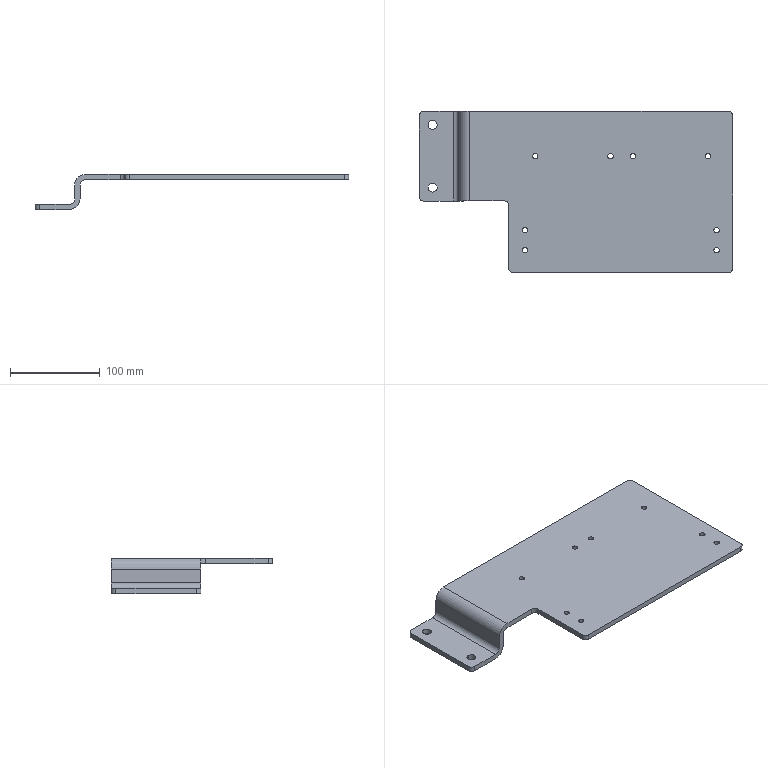Part | STEP file | J452-EBZ05-08-04-Part-1 | 1 solid | 42 faces | box 350 x 180 x 39.3 mm | volume 342916 mm3 | cylinder 30 | plane 12 | commonest cylinder face diameters 6 x16 10 x10 12 x2 24 x2